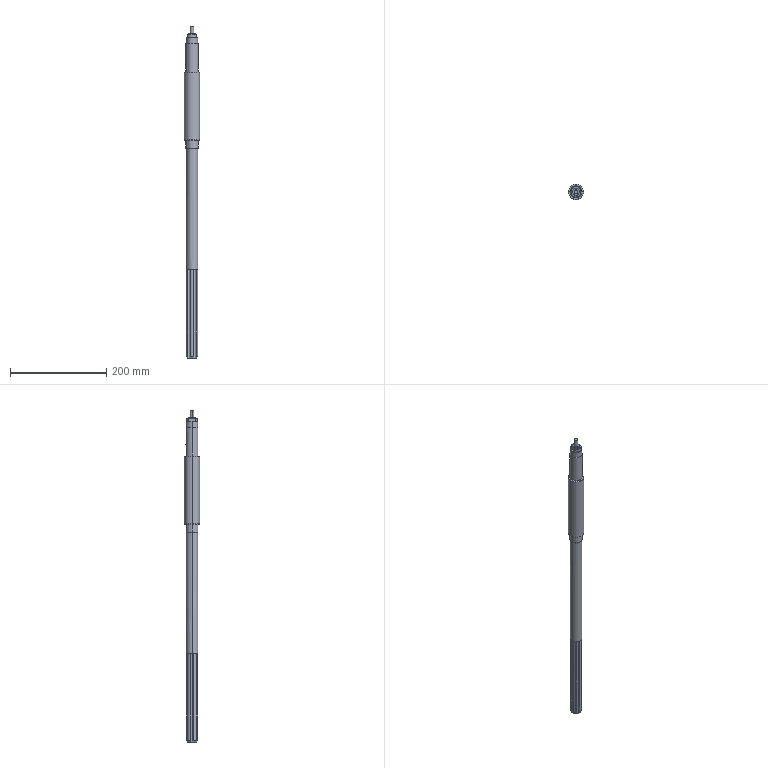Part | SolidWorks | features ICE 14, Chamfer 8, CirPattern 1, Extrusion 1 | 1 solid | 99 faces | box 32 x 32 x 689 mm | volume 345284 mm3 | plane 41 | cylinder 38 | cone 20 | commonest cylinder face diameters 24.5 x10 20 x7 24 x4 25 x4 3 x3 14 x3